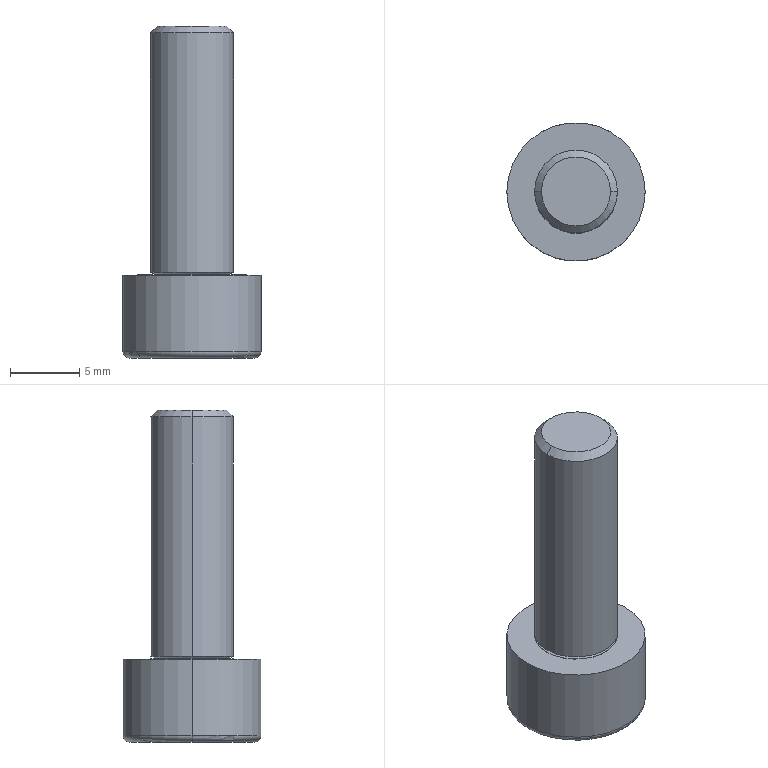Part | SolidWorks | features Attribute 1, Cut 1, Revolution 1 | 1 solid | 27 faces | box 10 x 10 x 24 mm | volume 921.395 mm3 | plane 11 | torus 6 | cylinder 6 | cone 4 | commonest cylinder face diameters 6 x4 10 x2
STEP:
#1=CARTESIAN_POINT('',(-2.613,0.,0.01));
#2=VERTEX_POINT('',#1);
#3=CARTESIAN_POINT('',(-2.593,0.,0.03));
#4=VERTEX_POINT('',#3);
#5=CARTESIAN_POINT('',(-2.613,0.,0.03));
#6=DIRECTION('',(0.,-1.,0.));
#7=DIRECTION('',(0.,0.,-1.));
#8=AXIS2_PLACEMENT_3D('',#5,#6,#7);
#9=CIRCLE('',#8,0.02);
#10=EDGE_CURVE('',#2,#4,#9,.T.);
#11=ORIENTED_EDGE('',*,*,#10,.T.);
#12=CARTESIAN_POINT('',(2.593,0.,0.03));
#13=VERTEX_POINT('',#12);
#14=CARTESIAN_POINT('',(0.,0.,0.03));
#15=DIRECTION('',(0.,0.,-1.));
#16=DIRECTION('',(-1.,0.,0.));
#17=AXIS2_PLACEMENT_3D('',#14,#15,#16);
#18=CIRCLE('',#17,2.593);
#19=EDGE_CURVE('',#4,#13,#18,.T.);
#20=ORIENTED_EDGE('',*,*,#19,.T.);
#21=CARTESIAN_POINT('',(2.613,0.,0.01));
#22=VERTEX_POINT('',#21);
#23=CARTESIAN_POINT('',(2.613,0.,0.03));
#24=DIRECTION('',(0.,1.,0.));
#25=DIRECTION('',(-1.,0.,0.));
#26=AXIS2_PLACEMENT_3D('',#23,#24,#25);
#27=CIRCLE('',#26,0.02);
#28=EDGE_CURVE('',#22,#13,#27,.T.);
#29=ORIENTED_EDGE('',*,*,#28,.F.);
#30=CARTESIAN_POINT('',(0.,0.,0.01));
#31=DIRECTION('',(0.,0.,-1.));
#32=DIRECTION('',(-1.,0.,0.));
#33=AXIS2_PLACEMENT_3D('',#30,#31,#32);
#34=CIRCLE('',#33,2.613);
#35=EDGE_CURVE('',#2,#22,#34,.T.);
#36=ORIENTED_EDGE('',*,*,#35,.F.);
#37=EDGE_LOOP('',(#11,#20,#29,#36));
#38=FACE_OUTER_BOUND('',#37,.T.);
#39=CARTESIAN_POINT('',(0.,0.,0.03));
#40=DIRECTION('',(0.,0.,-1.));
#41=DIRECTION('',(-1.,0.,0.));
#42=AXIS2_PLACEMENT_3D('',#39,#40,#41);
#43=TOROIDAL_SURFACE('',#42,2.613,0.02);
#44=ADVANCED_FACE('',(#38),#43,.F.);
#45=ORIENTED_EDGE('',*,*,#28,.T.);
#46=CARTESIAN_POINT('',(0.,0.,0.03));
#47=DIRECTION('',(0.,0.,-1.));
#48=DIRECTION('',(-1.,0.,0.));
#49=AXIS2_PLACEMENT_3D('',#46,#47,#48);
#50=CIRCLE('',#49,2.593);
#51=EDGE_CURVE('',#13,#4,#50,.T.);
#52=ORIENTED_EDGE('',*,*,#51,.T.);
#53=ORIENTED_EDGE('',*,*,#10,.F.);
#54=CARTESIAN_POINT('',(0.,0.,0.01));
#55=DIRECTION('',(0.,0.,-1.));
#56=DIRECTION('',(-1.,0.,0.));
#57=AXIS2_PLACEMENT_3D('',#54,#55,#56);
#58=CIRCLE('',#57,2.613);
#59=EDGE_CURVE('',#22,#2,#58,.T.);
#60=ORIENTED_EDGE('',*,*,#59,.F.);
#61=EDGE_LOOP('',(#45,#52,#53,#60));
#62=FACE_OUTER_BOUND('',#61,.T.);
#63=CARTESIAN_POINT('',(0.,0.,0.03));
#64=DIRECTION('',(0.,0.,-1.));
#65=DIRECTION('',(-1.,0.,0.));
#66=AXIS2_PLACEMENT_3D('',#63,#64,#65);
#67=TOROIDAL_SURFACE('',#66,2.613,0.02);
#68=ADVANCED_FACE('',(#62),#67,.F.);
#69=CARTESIAN_POINT('',(-2.5,0.,18.));
#70=VERTEX_POINT('',#69);
#71=CARTESIAN_POINT('',(2.5,0.,18.));
#72=VERTEX_POINT('',#71);
#73=CARTESIAN_POINT('',(0.,0.,18.));
#74=DIRECTION('',(0.,0.,-1.));
#75=DIRECTION('',(-1.,0.,0.));
#76=AXIS2_PLACEMENT_3D('',#73,#74,#75);
#77=CIRCLE('',#76,2.5);
#78=EDGE_CURVE('',#70,#72,#77,.T.);
#79=ORIENTED_EDGE('',*,*,#78,.T.);
#80=CARTESIAN_POINT('',(3.,0.,17.5));
#81=VERTEX_POINT('',#80);
#82=CARTESIAN_POINT('',(2.5,0.,18.));
#83=DIRECTION('',(0.7071,0.,-0.7071));
#84=VECTOR('',#83,1000.);
#85=LINE('',#82,#84);
#86=EDGE_CURVE('',#72,#81,#85,.T.);
#87=ORIENTED_EDGE('',*,*,#86,.T.);
#88=CARTESIAN_POINT('',(-3.,0.,17.5));
#89=VERTEX_POINT('',#88);
#90=CARTESIAN_POINT('',(0.,0.,17.5));
#91=DIRECTION('',(0.,0.,-1.));
#92=DIRECTION('',(-1.,0.,0.));
#93=AXIS2_PLACEMENT_3D('',#90,#91,#92);
#94=CIRCLE('',#93,3.);
#95=EDGE_CURVE('',#89,#81,#94,.T.);
#96=ORIENTED_EDGE('',*,*,#95,.F.);
#97=CARTESIAN_POINT('',(-2.5,0.,18.));
#98=DIRECTION('',(-0.7071,0.,-0.7071));
#99=VECTOR('',#98,1000.);
#100=LINE('',#97,#99);
#101=EDGE_CURVE('',#70,#89,#100,.T.);
#102=ORIENTED_EDGE('',*,*,#101,.F.);
#103=EDGE_LOOP('',(#79,#87,#96,#102));
#104=FACE_OUTER_BOUND('',#103,.T.);
#105=CARTESIAN_POINT('',(0.,0.,18.));
#106=DIRECTION('',(0.,0.,-1.));
#107=DIRECTION('',(-1.,0.,0.));
#108=AXIS2_PLACEMENT_3D('',#105,#106,#107);
#109=CONICAL_SURFACE('',#108,2.5,0.7854);
#110=ADVANCED_FACE('',(#104),#109,.T.);
#111=ORIENTED_EDGE('',*,*,#95,.T.);
#112=CARTESIAN_POINT('',(3.,0.,0.192));
#113=VERTEX_POINT('',#112);
#114=CARTESIAN_POINT('',(3.,0.,-10.585));
#115=DIRECTION('',(0.,0.,-1.));
#116=VECTOR('',#115,1000.);
#117=LINE('',#114,#116);
#118=EDGE_CURVE('',#81,#113,#117,.T.);
#119=ORIENTED_EDGE('',*,*,#118,.T.);
#120=CARTESIAN_POINT('',(-3.,0.,0.192));
#121=VERTEX_POINT('',#120);
#122=CARTESIAN_POINT('',(0.,0.,0.192));
#123=DIRECTION('',(0.,0.,-1.));
#124=DIRECTION('',(-1.,0.,0.));
#125=AXIS2_PLACEMENT_3D('',#122,#123,#124);
#126=CIRCLE('',#125,3.);
#127=EDGE_CURVE('',#121,#113,#126,.T.);
#128=ORIENTED_EDGE('',*,*,#127,.F.);
#129=CARTESIAN_POINT('',(-3.,0.,-10.585));
#130=DIRECTION('',(0.,0.,-1.));
#131=VECTOR('',#130,1000.);
#132=LINE('',#129,#131);
#133=EDGE_CURVE('',#89,#121,#132,.T.);
#134=ORIENTED_EDGE('',*,*,#133,.F.);
#135=EDGE_LOOP('',(#111,#119,#128,#134));
#136=FACE_OUTER_BOUND('',#135,.T.);
#137=CARTESIAN_POINT('',(0.,0.,-10.585));
#138=DIRECTION('',(0.,0.,-1.));
#139=DIRECTION('',(-1.,0.,0.));
#140=AXIS2_PLACEMENT_3D('',#137,#138,#139);
#141=CYLINDRICAL_SURFACE('',#140,3.);
#142=ADVANCED_FACE('',(#136),#141,.T.);
#143=CARTESIAN_POINT('',(-2.607,0.,0.04879));
#144=VERTEX_POINT('',#143);
#145=CARTESIAN_POINT('',(2.607,0.,0.04879));
#146=VERTEX_POINT('',#145);
#147=CARTESIAN_POINT('',(0.,0.,0.04879));
#148=DIRECTION('',(0.,0.,-1.));
#149=DIRECTION('',(-1.,0.,0.));
#150=AXIS2_PLACEMENT_3D('',#147,#148,#149);
#151=CIRCLE('',#150,2.607);
#152=EDGE_CURVE('',#144,#146,#151,.T.);
#153=ORIENTED_EDGE('',*,*,#152,.F.);
#154=CARTESIAN_POINT('',(-3.,0.,0.192));
#155=DIRECTION('',(-0.9397,0.,0.342));
#156=VECTOR('',#155,1000.);
#157=LINE('',#154,#156);
#158=EDGE_CURVE('',#144,#121,#157,.T.);
#159=ORIENTED_EDGE('',*,*,#158,.T.);
#160=ORIENTED_EDGE('',*,*,#127,.T.);
#161=CARTESIAN_POINT('',(3.,0.,0.192));
#162=DIRECTION('',(0.9397,0.,0.342));
#163=VECTOR('',#162,1000.);
#164=LINE('',#161,#163);
#165=EDGE_CURVE('',#146,#113,#164,.T.);
#166=ORIENTED_EDGE('',*,*,#165,.F.);
#167=EDGE_LOOP('',(#153,#159,#160,#166));
#168=FACE_OUTER_BOUND('',#167,.T.);
#169=CARTESIAN_POINT('',(0.,0.,0.192));
#170=DIRECTION('',(0.,0.,1.));
#171=DIRECTION('',(1.,0.,0.));
#172=AXIS2_PLACEMENT_3D('',#169,#170,#171);
#173=CONICAL_SURFACE('',#172,3.,1.222);
#174=ADVANCED_FACE('',(#168),#173,.T.);
#175=ORIENTED_EDGE('',*,*,#51,.F.);
#176=CARTESIAN_POINT('',(2.613,0.,0.03));
#177=DIRECTION('',(0.,1.,0.));
#178=DIRECTION('',(-1.,0.,0.));
#179=AXIS2_PLACEMENT_3D('',#176,#177,#178);
#180=CIRCLE('',#179,0.02);
#181=EDGE_CURVE('',#13,#146,#180,.T.);
#182=ORIENTED_EDGE('',*,*,#181,.T.);
#183=CARTESIAN_POINT('',(0.,0.,0.04879));
#184=DIRECTION('',(0.,0.,-1.));
#185=DIRECTION('',(-1.,0.,0.));
#186=AXIS2_PLACEMENT_3D('',#183,#184,#185);
#187=CIRCLE('',#186,2.607);
#188=EDGE_CURVE('',#146,#144,#187,.T.);
#189=ORIENTED_EDGE('',*,*,#188,.T.);
#190=CARTESIAN_POINT('',(-2.613,0.,0.03));
#191=DIRECTION('',(0.,-1.,0.));
#192=DIRECTION('',(0.,0.,-1.));
#193=AXIS2_PLACEMENT_3D('',#190,#191,#192);
#194=CIRCLE('',#193,0.02);
#195=EDGE_CURVE('',#4,#144,#194,.T.);
#196=ORIENTED_EDGE('',*,*,#195,.F.);
#197=EDGE_LOOP('',(#175,#182,#189,#196));
#198=FACE_OUTER_BOUND('',#197,.T.);
#199=CARTESIAN_POINT('',(0.,0.,0.03));
#200=DIRECTION('',(0.,0.,-1.));
#201=DIRECTION('',(-1.,0.,0.));
#202=AXIS2_PLACEMENT_3D('',#199,#200,#201);
#203=TOROIDAL_SURFACE('',#202,2.613,0.02);
#204=ADVANCED_FACE('',(#198),#203,.F.);
#205=CARTESIAN_POINT('',(-3.,0.,0.01));
#206=VERTEX_POINT('',#205);
#207=CARTESIAN_POINT('',(3.,0.,0.01));
#208=VERTEX_POINT('',#207);
#209=CARTESIAN_POINT('',(0.,0.,0.01));
#210=DIRECTION('',(0.,0.,-1.));
#211=DIRECTION('',(-1.,0.,0.));
#212=AXIS2_PLACEMENT_3D('',#209,#210,#211);
#213=CIRCLE('',#212,3.);
#214=EDGE_CURVE('',#206,#208,#213,.T.);
#215=ORIENTED_EDGE('',*,*,#214,.T.);
#216=CARTESIAN_POINT('',(3.,0.,0.));
#217=VERTEX_POINT('',#216);
#218=CARTESIAN_POINT('',(3.,0.,-10.585));
#219=DIRECTION('',(0.,0.,-1.));
#220=VECTOR('',#219,1000.);
#221=LINE('',#218,#220);
#222=EDGE_CURVE('',#208,#217,#221,.T.);
#223=ORIENTED_EDGE('',*,*,#222,.T.);
#224=CARTESIAN_POINT('',(-3.,0.,0.));
#225=VERTEX_POINT('',#224);
#226=CARTESIAN_POINT('',(0.,0.,0.));
#227=DIRECTION('',(0.,0.,-1.));
#228=DIRECTION('',(-1.,0.,0.));
#229=AXIS2_PLACEMENT_3D('',#226,#227,#228);
#230=CIRCLE('',#229,3.);
#231=EDGE_CURVE('',#225,#217,#230,.T.);
#232=ORIENTED_EDGE('',*,*,#231,.F.);
#233=CARTESIAN_POINT('',(-3.,0.,-10.585));
#234=DIRECTION('',(0.,0.,-1.));
#235=VECTOR('',#234,1000.);
#236=LINE('',#233,#235);
#237=EDGE_CURVE('',#206,#225,#236,.T.);
#238=ORIENTED_EDGE('',*,*,#237,.F.);
#239=EDGE_LOOP('',(#215,#223,#232,#238));
#240=FACE_OUTER_BOUND('',#239,.T.);
#241=CARTESIAN_POINT('',(0.,0.,-10.585));
#242=DIRECTION('',(0.,0.,-1.));
#243=DIRECTION('',(-1.,0.,0.));
#244=AXIS2_PLACEMENT_3D('',#241,#242,#243);
#245=CYLINDRICAL_SURFACE('',#244,3.);
#246=ADVANCED_FACE('',(#240),#245,.T.);
#247=CARTESIAN_POINT('',(-5.,0.,0.));
#248=VERTEX_POINT('',#247);
#249=CARTESIAN_POINT('',(5.,0.,0.));
#250=VERTEX_POINT('',#249);
#251=CARTESIAN_POINT('',(0.,0.,0.));
#252=DIRECTION('',(0.,0.,-1.));
#253=DIRECTION('',(-1.,0.,0.));
#254=AXIS2_PLACEMENT_3D('',#251,#252,#253);
#255=CIRCLE('',#254,5.);
#256=EDGE_CURVE('',#248,#250,#255,.T.);
#257=ORIENTED_EDGE('',*,*,#256,.T.);
#258=CARTESIAN_POINT('',(5.,0.,-5.5));
#259=VERTEX_POINT('',#258);
#260=CARTESIAN_POINT('',(5.,0.,-10.585));
#261=DIRECTION('',(0.,0.,-1.));
#262=VECTOR('',#261,1000.);
#263=LINE('',#260,#262);
#264=EDGE_CURVE('',#250,#259,#263,.T.);
#265=ORIENTED_EDGE('',*,*,#264,.T.);
#266=CARTESIAN_POINT('',(-5.,0.,-5.5));
#267=VERTEX_POINT('',#266);
#268=CARTESIAN_POINT('',(0.,0.,-5.5));
#269=DIRECTION('',(0.,0.,-1.));
#270=DIRECTION('',(-1.,0.,0.));
#271=AXIS2_PLACEMENT_3D('',#268,#269,#270);
#272=CIRCLE('',#271,5.);
#273=EDGE_CURVE('',#267,#259,#272,.T.);
#274=ORIENTED_EDGE('',*,*,#273,.F.);
#275=CARTESIAN_POINT('',(-5.,0.,-10.585));
#276=DIRECTION('',(0.,0.,-1.));
#277=VECTOR('',#276,1000.);
#278=LINE('',#275,#277);
#279=EDGE_CURVE('',#248,#267,#278,.T.);
#280=ORIENTED_EDGE('',*,*,#279,.F.);
#281=EDGE_LOOP('',(#257,#265,#274,#280));
#282=FACE_OUTER_BOUND('',#281,.T.);
#283=CARTESIAN_POINT('',(0.,0.,-10.585));
#284=DIRECTION('',(0.,0.,-1.));
#285=DIRECTION('',(-1.,0.,0.));
#286=AXIS2_PLACEMENT_3D('',#283,#284,#285);
#287=CYLINDRICAL_SURFACE('',#286,5.);
#288=ADVANCED_FACE('',(#282),#287,.T.);
#289=ORIENTED_EDGE('',*,*,#273,.T.);
#290=CARTESIAN_POINT('',(4.5,0.,-6.));
#291=VERTEX_POINT('',#290);
#292=CARTESIAN_POINT('',(4.5,0.,-5.5));
#293=DIRECTION('',(0.,1.,0.));
#294=DIRECTION('',(-1.,0.,0.));
#295=AXIS2_PLACEMENT_3D('',#292,#293,#294);
#296=CIRCLE('',#295,0.5);
#297=EDGE_CURVE('',#259,#291,#296,.T.);
#298=ORIENTED_EDGE('',*,*,#297,.T.);
#299=CARTESIAN_POINT('',(-4.5,0.,-6.));
#300=VERTEX_POINT('',#299);
#301=CARTESIAN_POINT('',(0.,0.,-6.));
#302=DIRECTION('',(0.,0.,-1.));
#303=DIRECTION('',(-1.,0.,0.));
#304=AXIS2_PLACEMENT_3D('',#301,#302,#303);
#305=CIRCLE('',#304,4.5);
#306=EDGE_CURVE('',#300,#291,#305,.T.);
#307=ORIENTED_EDGE('',*,*,#306,.F.);
#308=CARTESIAN_POINT('',(-4.5,0.,-5.5));
#309=DIRECTION('',(0.,-1.,0.));
#310=DIRECTION('',(0.,0.,-1.));
#311=AXIS2_PLACEMENT_3D('',#308,#309,#310);
#312=CIRCLE('',#311,0.5);
#313=EDGE_CURVE('',#267,#300,#312,.T.);
#314=ORIENTED_EDGE('',*,*,#313,.F.);
#315=EDGE_LOOP('',(#289,#298,#307,#314));
#316=FACE_OUTER_BOUND('',#315,.T.);
#317=CARTESIAN_POINT('',(0.,0.,-5.5));
#318=DIRECTION('',(0.,0.,-1.));
#319=DIRECTION('',(-1.,0.,0.));
#320=AXIS2_PLACEMENT_3D('',#317,#318,#319);
#321=TOROIDAL_SURFACE('',#320,4.5,0.5);
#322=ADVANCED_FACE('',(#316),#321,.T.);
#323=ORIENTED_EDGE('',*,*,#297,.F.);
#324=CARTESIAN_POINT('',(0.,0.,-5.5));
#325=DIRECTION('',(0.,0.,-1.));
#326=DIRECTION('',(-1.,0.,0.));
#327=AXIS2_PLACEMENT_3D('',#324,#325,#326);
#328=CIRCLE('',#327,5.);
#329=EDGE_CURVE('',#259,#267,#328,.T.);
#330=ORIENTED_EDGE('',*,*,#329,.T.);
#331=ORIENTED_EDGE('',*,*,#313,.T.);
#332=CARTESIAN_POINT('',(0.,0.,-6.));
#333=DIRECTION('',(0.,0.,-1.));
#334=DIRECTION('',(-1.,0.,0.));
#335=AXIS2_PLACEMENT_3D('',#332,#333,#334);
#336=CIRCLE('',#335,4.5);
#337=EDGE_CURVE('',#291,#300,#336,.T.);
#338=ORIENTED_EDGE('',*,*,#337,.F.);
#339=EDGE_LOOP('',(#323,#330,#331,#338));
#340=FACE_OUTER_BOUND('',#339,.T.);
#341=CARTESIAN_POINT('',(0.,0.,-5.5));
#342=DIRECTION('',(0.,0.,-1.));
#343=DIRECTION('',(-1.,0.,0.));
#344=AXIS2_PLACEMENT_3D('',#341,#342,#343);
#345=TOROIDAL_SURFACE('',#344,4.5,0.5);
#346=ADVANCED_FACE('',(#340),#345,.T.);
#347=ORIENTED_EDGE('',*,*,#264,.F.);
#348=CARTESIAN_POINT('',(0.,0.,0.));
#349=DIRECTION('',(0.,0.,-1.));
#350=DIRECTION('',(-1.,0.,0.));
#351=AXIS2_PLACEMENT_3D('',#348,#349,#350);
#352=CIRCLE('',#351,5.);
#353=EDGE_CURVE('',#250,#248,#352,.T.);
#354=ORIENTED_EDGE('',*,*,#353,.T.);
#355=ORIENTED_EDGE('',*,*,#279,.T.);
#356=ORIENTED_EDGE('',*,*,#329,.F.);
#357=EDGE_LOOP('',(#347,#354,#355,#356));
#358=FACE_OUTER_BOUND('',#357,.T.);
#359=CARTESIAN_POINT('',(0.,0.,-10.585));
#360=DIRECTION('',(0.,0.,-1.));
#361=DIRECTION('',(-1.,0.,0.));
#362=AXIS2_PLACEMENT_3D('',#359,#360,#361);
#363=CYLINDRICAL_SURFACE('',#362,5.);
#364=ADVANCED_FACE('',(#358),#363,.T.);
#365=ORIENTED_EDGE('',*,*,#256,.F.);
#366=ORIENTED_EDGE('',*,*,#353,.F.);
#367=EDGE_LOOP('',(#365,#366));
#368=FACE_OUTER_BOUND('',#367,.T.);
#369=ORIENTED_EDGE('',*,*,#231,.T.);
#370=CARTESIAN_POINT('',(0.,0.,0.));
#371=DIRECTION('',(0.,0.,-1.));
#372=DIRECTION('',(-1.,0.,0.));
#373=AXIS2_PLACEMENT_3D('',#370,#371,#372);
#374=CIRCLE('',#373,3.);
#375=EDGE_CURVE('',#217,#225,#374,.T.);
#376=ORIENTED_EDGE('',*,*,#375,.T.);
#377=EDGE_LOOP('',(#369,#376));
#378=FACE_BOUND('',#377,.T.);
#379=CARTESIAN_POINT('',(-5.,0.,0.));
#380=DIRECTION('',(0.,0.,-1.));
#381=DIRECTION('',(-1.,0.,0.));
#382=AXIS2_PLACEMENT_3D('',#379,#380,#381);
#383=PLANE('',#382);
#384=ADVANCED_FACE('',(#368,#378),#383,.F.);
#385=ORIENTED_EDGE('',*,*,#222,.F.);
#386=CARTESIAN_POINT('',(0.,0.,0.01));
#387=DIRECTION('',(0.,0.,-1.));
#388=DIRECTION('',(-1.,0.,0.));
#389=AXIS2_PLACEMENT_3D('',#386,#387,#388);
#390=CIRCLE('',#389,3.);
#391=EDGE_CURVE('',#208,#206,#390,.T.);
#392=ORIENTED_EDGE('',*,*,#391,.T.);
#393=ORIENTED_EDGE('',*,*,#237,.T.);
#394=ORIENTED_EDGE('',*,*,#375,.F.);
#395=EDGE_LOOP('',(#385,#392,#393,#394));
#396=FACE_OUTER_BOUND('',#395,.T.);
#397=CARTESIAN_POINT('',(0.,0.,-10.585));
#398=DIRECTION('',(0.,0.,-1.));
#399=DIRECTION('',(-1.,0.,0.));
#400=AXIS2_PLACEMENT_3D('',#397,#398,#399);
#401=CYLINDRICAL_SURFACE('',#400,3.);
#402=ADVANCED_FACE('',(#396),#401,.T.);
#403=ORIENTED_EDGE('',*,*,#214,.F.);
#404=ORIENTED_EDGE('',*,*,#391,.F.);
#405=EDGE_LOOP('',(#403,#404));
#406=FACE_OUTER_BOUND('',#405,.T.);
#407=ORIENTED_EDGE('',*,*,#35,.T.);
#408=ORIENTED_EDGE('',*,*,#59,.T.);
#409=EDGE_LOOP('',(#407,#408));
#410=FACE_BOUND('',#409,.T.);
#411=CARTESIAN_POINT('',(-3.,0.,0.01));
#412=DIRECTION('',(0.,0.,-1.));
#413=DIRECTION('',(-1.,0.,0.));
#414=AXIS2_PLACEMENT_3D('',#411,#412,#413);
#415=PLANE('',#414);
#416=ADVANCED_FACE('',(#406,#410),#415,.F.);
#417=ORIENTED_EDGE('',*,*,#19,.F.);
#418=ORIENTED_EDGE('',*,*,#195,.T.);
#419=ORIENTED_EDGE('',*,*,#152,.T.);
#420=ORIENTED_EDGE('',*,*,#181,.F.);
#421=EDGE_LOOP('',(#417,#418,#419,#420));
#422=FACE_OUTER_BOUND('',#421,.T.);
#423=CARTESIAN_POINT('',(0.,0.,0.03));
#424=DIRECTION('',(0.,0.,-1.));
#425=DIRECTION('',(-1.,0.,0.));
#426=AXIS2_PLACEMENT_3D('',#423,#424,#425);
#427=TOROIDAL_SURFACE('',#426,2.613,0.02);
#428=ADVANCED_FACE('',(#422),#427,.F.);
#429=ORIENTED_EDGE('',*,*,#158,.F.);
#430=ORIENTED_EDGE('',*,*,#188,.F.);
#431=ORIENTED_EDGE('',*,*,#165,.T.);
#432=CARTESIAN_POINT('',(0.,0.,0.192));
#433=DIRECTION('',(0.,0.,-1.));
#434=DIRECTION('',(-1.,0.,0.));
#435=AXIS2_PLACEMENT_3D('',#432,#433,#434);
#436=CIRCLE('',#435,3.);
#437=EDGE_CURVE('',#113,#121,#436,.T.);
#438=ORIENTED_EDGE('',*,*,#437,.T.);
#439=EDGE_LOOP('',(#429,#430,#431,#438));
#440=FACE_OUTER_BOUND('',#439,.T.);
#441=CARTESIAN_POINT('',(0.,0.,0.192));
#442=DIRECTION('',(0.,0.,1.));
#443=DIRECTION('',(1.,0.,0.));
#444=AXIS2_PLACEMENT_3D('',#441,#442,#443);
#445=CONICAL_SURFACE('',#444,3.,1.222);
#446=ADVANCED_FACE('',(#440),#445,.T.);
#447=ORIENTED_EDGE('',*,*,#118,.F.);
#448=CARTESIAN_POINT('',(0.,0.,17.5));
#449=DIRECTION('',(0.,0.,-1.));
#450=DIRECTION('',(-1.,0.,0.));
#451=AXIS2_PLACEMENT_3D('',#448,#449,#450);
#452=CIRCLE('',#451,3.);
#453=EDGE_CURVE('',#81,#89,#452,.T.);
#454=ORIENTED_EDGE('',*,*,#453,.T.);
#455=ORIENTED_EDGE('',*,*,#133,.T.);
#456=ORIENTED_EDGE('',*,*,#437,.F.);
#457=EDGE_LOOP('',(#447,#454,#455,#456));
#458=FACE_OUTER_BOUND('',#457,.T.);
#459=CARTESIAN_POINT('',(0.,0.,-10.585));
#460=DIRECTION('',(0.,0.,-1.));
#461=DIRECTION('',(-1.,0.,0.));
#462=AXIS2_PLACEMENT_3D('',#459,#460,#461);
#463=CYLINDRICAL_SURFACE('',#462,3.);
#464=ADVANCED_FACE('',(#458),#463,.T.);
#465=ORIENTED_EDGE('',*,*,#86,.F.);
#466=CARTESIAN_POINT('',(0.,0.,18.));
#467=DIRECTION('',(0.,0.,-1.));
#468=DIRECTION('',(-1.,0.,0.));
#469=AXIS2_PLACEMENT_3D('',#466,#467,#468);
#470=CIRCLE('',#469,2.5);
#471=EDGE_CURVE('',#72,#70,#470,.T.);
#472=ORIENTED_EDGE('',*,*,#471,.T.);
#473=ORIENTED_EDGE('',*,*,#101,.T.);
#474=ORIENTED_EDGE('',*,*,#453,.F.);
#475=EDGE_LOOP('',(#465,#472,#473,#474));
#476=FACE_OUTER_BOUND('',#475,.T.);
#477=CARTESIAN_POINT('',(0.,0.,18.));
#478=DIRECTION('',(0.,0.,-1.));
#479=DIRECTION('',(-1.,0.,0.));
#480=AXIS2_PLACEMENT_3D('',#477,#478,#479);
#481=CONICAL_SURFACE('',#480,2.5,0.7854);
#482=ADVANCED_FACE('',(#476),#481,.T.);
#483=ORIENTED_EDGE('',*,*,#78,.F.);
#484=ORIENTED_EDGE('',*,*,#471,.F.);
#485=EDGE_LOOP('',(#483,#484));
#486=FACE_OUTER_BOUND('',#485,.T.);
#487=CARTESIAN_POINT('',(-2.5,0.,18.));
#488=DIRECTION('',(0.,0.,-1.));
#489=DIRECTION('',(-1.,0.,0.));
#490=AXIS2_PLACEMENT_3D('',#487,#488,#489);
#491=PLANE('',#490);
#492=ADVANCED_FACE('',(#486),#491,.F.);
#493=CARTESIAN_POINT('',(2.887,0.,-6.));
#494=VERTEX_POINT('',#493);
#495=CARTESIAN_POINT('',(1.443,-2.5,-6.));
#496=VERTEX_POINT('',#495);
#497=CARTESIAN_POINT('',(2.887,0.,-6.));
#498=DIRECTION('',(-0.5,-0.866,0.));
#499=VECTOR('',#498,1000.);
#500=LINE('',#497,#499);
#501=EDGE_CURVE('',#494,#496,#500,.T.);
#502=ORIENTED_EDGE('',*,*,#501,.F.);
#503=CARTESIAN_POINT('',(1.443,2.5,-6.));
#504=VERTEX_POINT('',#503);
#505=CARTESIAN_POINT('',(1.443,2.5,-6.));
#506=DIRECTION('',(0.5,-0.866,0.));
#507=VECTOR('',#506,1000.);
#508=LINE('',#505,#507);
#509=EDGE_CURVE('',#504,#494,#508,.T.);
#510=ORIENTED_EDGE('',*,*,#509,.F.);
#511=CARTESIAN_POINT('',(-1.443,2.5,-6.));
#512=VERTEX_POINT('',#511);
#513=CARTESIAN_POINT('',(-1.443,2.5,-6.));
#514=DIRECTION('',(1.,0.,0.));
#515=VECTOR('',#514,1000.);
#516=LINE('',#513,#515);
#517=EDGE_CURVE('',#512,#504,#516,.T.);
#518=ORIENTED_EDGE('',*,*,#517,.F.);
#519=CARTESIAN_POINT('',(-2.887,0.,-6.));
#520=VERTEX_POINT('',#519);
#521=CARTESIAN_POINT('',(-2.887,0.,-6.));
#522=DIRECTION('',(0.5,0.866,0.));
#523=VECTOR('',#522,1000.);
#524=LINE('',#521,#523);
#525=EDGE_CURVE('',#520,#512,#524,.T.);
#526=ORIENTED_EDGE('',*,*,#525,.F.);
#527=CARTESIAN_POINT('',(-1.443,-2.5,-6.));
#528=VERTEX_POINT('',#527);
#529=CARTESIAN_POINT('',(-1.443,-2.5,-6.));
#530=DIRECTION('',(-0.5,0.866,0.));
#531=VECTOR('',#530,1000.);
#532=LINE('',#529,#531);
#533=EDGE_CURVE('',#528,#520,#532,.T.);
#534=ORIENTED_EDGE('',*,*,#533,.F.);
#535=CARTESIAN_POINT('',(1.443,-2.5,-6.));
#536=DIRECTION('',(-1.,0.,0.));
#537=VECTOR('',#536,1000.);
#538=LINE('',#535,#537);
#539=EDGE_CURVE('',#496,#528,#538,.T.);
#540=ORIENTED_EDGE('',*,*,#539,.F.);
#541=EDGE_LOOP('',(#502,#510,#518,#526,#534,#540));
#542=FACE_BOUND('',#541,.T.);
#543=ORIENTED_EDGE('',*,*,#306,.T.);
#544=ORIENTED_EDGE('',*,*,#337,.T.);
#545=EDGE_LOOP('',(#543,#544));
#546=FACE_OUTER_BOUND('',#545,.T.);
#547=CARTESIAN_POINT('',(0.,0.,-6.));
#548=DIRECTION('',(0.,0.,1.));
#549=DIRECTION('',(1.,0.,0.));
#550=AXIS2_PLACEMENT_3D('',#547,#548,#549);
#551=PLANE('',#550);
#552=ADVANCED_FACE('',(#542,#546),#551,.F.);
#553=ORIENTED_EDGE('',*,*,#509,.T.);
#554=CARTESIAN_POINT('',(2.887,0.,-3.5));
#555=VERTEX_POINT('',#554);
#556=CARTESIAN_POINT('',(2.887,0.,-3.5));
#557=DIRECTION('',(0.,0.,-1.));
#558=VECTOR('',#557,1000.);
#559=LINE('',#556,#558);
#560=EDGE_CURVE('',#555,#494,#559,.T.);
#561=ORIENTED_EDGE('',*,*,#560,.F.);
#562=CARTESIAN_POINT('',(1.443,2.5,-3.5));
#563=VERTEX_POINT('',#562);
#564=CARTESIAN_POINT('',(1.443,2.5,-3.5));
#565=DIRECTION('',(0.5,-0.866,0.));
#566=VECTOR('',#565,1000.);
#567=LINE('',#564,#566);
#568=EDGE_CURVE('',#563,#555,#567,.T.);
#569=ORIENTED_EDGE('',*,*,#568,.F.);
#570=CARTESIAN_POINT('',(1.443,2.5,-3.5));
#571=DIRECTION('',(0.,0.,-1.));
#572=VECTOR('',#571,1000.);
#573=LINE('',#570,#572);
#574=EDGE_CURVE('',#563,#504,#573,.T.);
#575=ORIENTED_EDGE('',*,*,#574,.T.);
#576=EDGE_LOOP('',(#553,#561,#569,#575));
#577=FACE_OUTER_BOUND('',#576,.T.);
#578=CARTESIAN_POINT('',(1.443,2.5,-3.5));
#579=DIRECTION('',(0.866,0.5,0.));
#580=DIRECTION('',(-0.5,0.866,0.));
#581=AXIS2_PLACEMENT_3D('',#578,#579,#580);
#582=PLANE('',#581);
#583=ADVANCED_FACE('',(#577),#582,.F.);
#584=ORIENTED_EDGE('',*,*,#517,.T.);
#585=ORIENTED_EDGE('',*,*,#574,.F.);
#586=CARTESIAN_POINT('',(-1.443,2.5,-3.5));
#587=VERTEX_POINT('',#586);
#588=CARTESIAN_POINT('',(-1.443,2.5,-3.5));
#589=DIRECTION('',(1.,0.,0.));
#590=VECTOR('',#589,1000.);
#591=LINE('',#588,#590);
#592=EDGE_CURVE('',#587,#563,#591,.T.);
#593=ORIENTED_EDGE('',*,*,#592,.F.);
#594=CARTESIAN_POINT('',(-1.443,2.5,-3.5));
#595=DIRECTION('',(0.,0.,-1.));
#596=VECTOR('',#595,1000.);
#597=LINE('',#594,#596);
#598=EDGE_CURVE('',#587,#512,#597,.T.);
#599=ORIENTED_EDGE('',*,*,#598,.T.);
#600=EDGE_LOOP('',(#584,#585,#593,#599));
#601=FACE_OUTER_BOUND('',#600,.T.);
#602=CARTESIAN_POINT('',(-1.443,2.5,-3.5));
#603=DIRECTION('',(0.,1.,0.));
#604=DIRECTION('',(-1.,0.,0.));
#605=AXIS2_PLACEMENT_3D('',#602,#603,#604);
#606=PLANE('',#605);
#607=ADVANCED_FACE('',(#601),#606,.F.);
#608=ORIENTED_EDGE('',*,*,#525,.T.);
#609=ORIENTED_EDGE('',*,*,#598,.F.);
#610=CARTESIAN_POINT('',(-2.887,0.,-3.5));
#611=VERTEX_POINT('',#610);
#612=CARTESIAN_POINT('',(-2.887,0.,-3.5));
#613=DIRECTION('',(0.5,0.866,0.));
#614=VECTOR('',#613,1000.);
#615=LINE('',#612,#614);
#616=EDGE_CURVE('',#611,#587,#615,.T.);
#617=ORIENTED_EDGE('',*,*,#616,.F.);
#618=CARTESIAN_POINT('',(-2.887,0.,-3.5));
#619=DIRECTION('',(0.,0.,-1.));
#620=VECTOR('',#619,1000.);
#621=LINE('',#618,#620);
#622=EDGE_CURVE('',#611,#520,#621,.T.);
#623=ORIENTED_EDGE('',*,*,#622,.T.);
#624=EDGE_LOOP('',(#608,#609,#617,#623));
#625=FACE_OUTER_BOUND('',#624,.T.);
#626=CARTESIAN_POINT('',(-2.887,0.,-3.5));
#627=DIRECTION('',(-0.866,0.5,0.));
#628=DIRECTION('',(-0.5,-0.866,0.));
#629=AXIS2_PLACEMENT_3D('',#626,#627,#628);
#630=PLANE('',#629);
#631=ADVANCED_FACE('',(#625),#630,.F.);
#632=ORIENTED_EDGE('',*,*,#533,.T.);
#633=ORIENTED_EDGE('',*,*,#622,.F.);
#634=CARTESIAN_POINT('',(-1.443,-2.5,-3.5));
#635=VERTEX_POINT('',#634);
#636=CARTESIAN_POINT('',(-1.443,-2.5,-3.5));
#637=DIRECTION('',(-0.5,0.866,0.));
#638=VECTOR('',#637,1000.);
#639=LINE('',#636,#638);
#640=EDGE_CURVE('',#635,#611,#639,.T.);
#641=ORIENTED_EDGE('',*,*,#640,.F.);
#642=CARTESIAN_POINT('',(-1.443,-2.5,-3.5));
#643=DIRECTION('',(0.,0.,-1.));
#644=VECTOR('',#643,1000.);
#645=LINE('',#642,#644);
#646=EDGE_CURVE('',#635,#528,#645,.T.);
#647=ORIENTED_EDGE('',*,*,#646,.T.);
#648=EDGE_LOOP('',(#632,#633,#641,#647));
#649=FACE_OUTER_BOUND('',#648,.T.);
#650=CARTESIAN_POINT('',(-1.443,-2.5,-3.5));
#651=DIRECTION('',(-0.866,-0.5,0.));
#652=DIRECTION('',(0.5,-0.866,0.));
#653=AXIS2_PLACEMENT_3D('',#650,#651,#652);
#654=PLANE('',#653);
#655=ADVANCED_FACE('',(#649),#654,.F.);
#656=ORIENTED_EDGE('',*,*,#539,.T.);
#657=ORIENTED_EDGE('',*,*,#646,.F.);
#658=CARTESIAN_POINT('',(1.443,-2.5,-3.5));
#659=VERTEX_POINT('',#658);
#660=CARTESIAN_POINT('',(1.443,-2.5,-3.5));
#661=DIRECTION('',(-1.,0.,0.));
#662=VECTOR('',#661,1000.);
#663=LINE('',#660,#662);
#664=EDGE_CURVE('',#659,#635,#663,.T.);
#665=ORIENTED_EDGE('',*,*,#664,.F.);
#666=CARTESIAN_POINT('',(1.443,-2.5,-3.5));
#667=DIRECTION('',(0.,0.,-1.));
#668=VECTOR('',#667,1000.);
#669=LINE('',#666,#668);
#670=EDGE_CURVE('',#659,#496,#669,.T.);
#671=ORIENTED_EDGE('',*,*,#670,.T.);
#672=EDGE_LOOP('',(#656,#657,#665,#671));
#673=FACE_OUTER_BOUND('',#672,.T.);
#674=CARTESIAN_POINT('',(1.443,-2.5,-3.5));
#675=DIRECTION('',(0.,-1.,0.));
#676=DIRECTION('',(0.,0.,-1.));
#677=AXIS2_PLACEMENT_3D('',#674,#675,#676);
#678=PLANE('',#677);
#679=ADVANCED_FACE('',(#673),#678,.F.);
#680=ORIENTED_EDGE('',*,*,#501,.T.);
#681=ORIENTED_EDGE('',*,*,#670,.F.);
#682=CARTESIAN_POINT('',(2.887,0.,-3.5));
#683=DIRECTION('',(-0.5,-0.866,0.));
#684=VECTOR('',#683,1000.);
#685=LINE('',#682,#684);
#686=EDGE_CURVE('',#555,#659,#685,.T.);
#687=ORIENTED_EDGE('',*,*,#686,.F.);
#688=ORIENTED_EDGE('',*,*,#560,.T.);
#689=EDGE_LOOP('',(#680,#681,#687,#688));
#690=FACE_OUTER_BOUND('',#689,.T.);
#691=CARTESIAN_POINT('',(2.887,0.,-3.5));
#692=DIRECTION('',(0.866,-0.5,0.));
#693=DIRECTION('',(0.5,0.866,0.));
#694=AXIS2_PLACEMENT_3D('',#691,#692,#693);
#695=PLANE('',#694);
#696=ADVANCED_FACE('',(#690),#695,.F.);
#697=ORIENTED_EDGE('',*,*,#568,.T.);
#698=ORIENTED_EDGE('',*,*,#686,.T.);
#699=ORIENTED_EDGE('',*,*,#664,.T.);
#700=ORIENTED_EDGE('',*,*,#640,.T.);
#701=ORIENTED_EDGE('',*,*,#616,.T.);
#702=ORIENTED_EDGE('',*,*,#592,.T.);
#703=EDGE_LOOP('',(#697,#698,#699,#700,#701,#702));
#704=FACE_OUTER_BOUND('',#703,.T.);
#705=CARTESIAN_POINT('',(1.443,2.5,-3.5));
#706=DIRECTION('',(0.,0.,1.));
#707=DIRECTION('',(1.,0.,0.));
#708=AXIS2_PLACEMENT_3D('',#705,#706,#707);
#709=PLANE('',#708);
#710=ADVANCED_FACE('',(#704),#709,.F.);
#711=CLOSED_SHELL('',(#44,#68,#110,#142,#174,#204,#246,#288,#322,#346,#364,#384,#402,#416,#428,#446,#464,#482,#492,#552,#583,#607,#631,#655,#679,#696,#710));
#712=MANIFOLD_SOLID_BREP('',#711);
#713=CARTESIAN_POINT('',(0.,0.,0.));
#714=DIRECTION('',(0.,0.,1.));
#715=DIRECTION('',(1.,0.,0.));
#716=AXIS2_PLACEMENT_3D('',#713,#714,#715);
#717=(LENGTH_UNIT()NAMED_UNIT(*)SI_UNIT(.MILLI.,.METRE.));
#718=UNCERTAINTY_MEASURE_WITH_UNIT(LENGTH_MEASURE(0.00001),#717,'','');
#719=(NAMED_UNIT(*)PLANE_ANGLE_UNIT()SI_UNIT($,.RADIAN.));
#720=(NAMED_UNIT(*)SI_UNIT($,.STERADIAN.)SOLID_ANGLE_UNIT());
#721=(GEOMETRIC_REPRESENTATION_CONTEXT(3)GLOBAL_UNCERTAINTY_ASSIGNED_CONTEXT((#718))GLOBAL_UNIT_ASSIGNED_CONTEXT((#717,#719,#720))REPRESENTATION_CONTEXT('',''));
#722=ADVANCED_BREP_SHAPE_REPRESENTATION('',(#712,#716),#721);